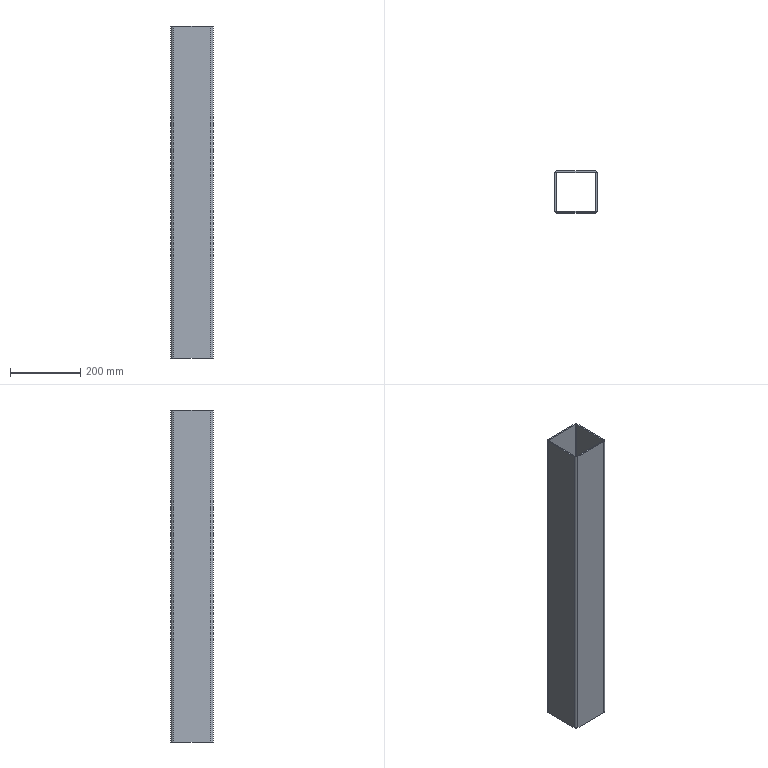Part | SolidWorks | features ICE 1, LibraryFeature 1 | 1 solid | 18 faces | box 120 x 120 x 945 mm | volume 1714983 mm3 | plane 10 | cylinder 8 | commonest cylinder face diameters 8 x4 16 x4
STEP:
#1=CARTESIAN_POINT('',(52.,60.,-472.5));
#2=VERTEX_POINT('',#1);
#3=CARTESIAN_POINT('',(-52.,60.,-472.5));
#4=VERTEX_POINT('',#3);
#5=CARTESIAN_POINT('',(0.,60.,-472.5));
#6=DIRECTION('',(-1.,0.,0.));
#7=VECTOR('',#6,1000.);
#8=LINE('',#5,#7);
#9=EDGE_CURVE('',#2,#4,#8,.T.);
#10=ORIENTED_EDGE('',*,*,#9,.T.);
#11=CARTESIAN_POINT('',(-52.,60.,472.5));
#12=VERTEX_POINT('',#11);
#13=CARTESIAN_POINT('',(-52.,60.,472.5));
#14=DIRECTION('',(0.,0.,-1.));
#15=VECTOR('',#14,1000.);
#16=LINE('',#13,#15);
#17=EDGE_CURVE('',#12,#4,#16,.T.);
#18=ORIENTED_EDGE('',*,*,#17,.F.);
#19=CARTESIAN_POINT('',(52.,60.,472.5));
#20=VERTEX_POINT('',#19);
#21=CARTESIAN_POINT('',(0.,60.,472.5));
#22=DIRECTION('',(-1.,0.,0.));
#23=VECTOR('',#22,1000.);
#24=LINE('',#21,#23);
#25=EDGE_CURVE('',#20,#12,#24,.T.);
#26=ORIENTED_EDGE('',*,*,#25,.F.);
#27=CARTESIAN_POINT('',(52.,60.,472.5));
#28=DIRECTION('',(0.,0.,-1.));
#29=VECTOR('',#28,1000.);
#30=LINE('',#27,#29);
#31=EDGE_CURVE('',#20,#2,#30,.T.);
#32=ORIENTED_EDGE('',*,*,#31,.T.);
#33=EDGE_LOOP('',(#10,#18,#26,#32));
#34=FACE_OUTER_BOUND('',#33,.T.);
#35=CARTESIAN_POINT('',(0.,60.,472.5));
#36=DIRECTION('',(0.,-1.,0.));
#37=DIRECTION('',(0.,0.,-1.));
#38=AXIS2_PLACEMENT_3D('',#35,#36,#37);
#39=PLANE('',#38);
#40=ADVANCED_FACE('',(#34),#39,.F.);
#41=CARTESIAN_POINT('',(-60.,52.,-472.5));
#42=VERTEX_POINT('',#41);
#43=CARTESIAN_POINT('',(-52.,52.,-472.5));
#44=DIRECTION('',(0.,0.,1.));
#45=DIRECTION('',(1.,0.,0.));
#46=AXIS2_PLACEMENT_3D('',#43,#44,#45);
#47=CIRCLE('',#46,8.);
#48=EDGE_CURVE('',#4,#42,#47,.T.);
#49=ORIENTED_EDGE('',*,*,#48,.T.);
#50=CARTESIAN_POINT('',(-60.,52.,472.5));
#51=VERTEX_POINT('',#50);
#52=CARTESIAN_POINT('',(-60.,52.,472.5));
#53=DIRECTION('',(0.,0.,-1.));
#54=VECTOR('',#53,1000.);
#55=LINE('',#52,#54);
#56=EDGE_CURVE('',#51,#42,#55,.T.);
#57=ORIENTED_EDGE('',*,*,#56,.F.);
#58=CARTESIAN_POINT('',(-52.,52.,472.5));
#59=DIRECTION('',(0.,0.,1.));
#60=DIRECTION('',(1.,0.,0.));
#61=AXIS2_PLACEMENT_3D('',#58,#59,#60);
#62=CIRCLE('',#61,8.);
#63=EDGE_CURVE('',#12,#51,#62,.T.);
#64=ORIENTED_EDGE('',*,*,#63,.F.);
#65=ORIENTED_EDGE('',*,*,#17,.T.);
#66=EDGE_LOOP('',(#49,#57,#64,#65));
#67=FACE_OUTER_BOUND('',#66,.T.);
#68=CARTESIAN_POINT('',(-52.,52.,472.5));
#69=DIRECTION('',(0.,0.,-1.));
#70=DIRECTION('',(-1.,0.,0.));
#71=AXIS2_PLACEMENT_3D('',#68,#69,#70);
#72=CYLINDRICAL_SURFACE('',#71,8.);
#73=ADVANCED_FACE('',(#67),#72,.T.);
#74=CARTESIAN_POINT('',(-60.,-52.,-472.5));
#75=VERTEX_POINT('',#74);
#76=CARTESIAN_POINT('',(-60.,0.,-472.5));
#77=DIRECTION('',(0.,1.,0.));
#78=VECTOR('',#77,1000.);
#79=LINE('',#76,#78);
#80=EDGE_CURVE('',#75,#42,#79,.T.);
#81=ORIENTED_EDGE('',*,*,#80,.F.);
#82=CARTESIAN_POINT('',(-60.,-52.,472.5));
#83=VERTEX_POINT('',#82);
#84=CARTESIAN_POINT('',(-60.,-52.,472.5));
#85=DIRECTION('',(0.,0.,-1.));
#86=VECTOR('',#85,1000.);
#87=LINE('',#84,#86);
#88=EDGE_CURVE('',#83,#75,#87,.T.);
#89=ORIENTED_EDGE('',*,*,#88,.F.);
#90=CARTESIAN_POINT('',(-60.,0.,472.5));
#91=DIRECTION('',(0.,1.,0.));
#92=VECTOR('',#91,1000.);
#93=LINE('',#90,#92);
#94=EDGE_CURVE('',#83,#51,#93,.T.);
#95=ORIENTED_EDGE('',*,*,#94,.T.);
#96=ORIENTED_EDGE('',*,*,#56,.T.);
#97=EDGE_LOOP('',(#81,#89,#95,#96));
#98=FACE_OUTER_BOUND('',#97,.T.);
#99=CARTESIAN_POINT('',(-60.,0.,472.5));
#100=DIRECTION('',(-1.,0.,0.));
#101=DIRECTION('',(0.,0.,1.));
#102=AXIS2_PLACEMENT_3D('',#99,#100,#101);
#103=PLANE('',#102);
#104=ADVANCED_FACE('',(#98),#103,.T.);
#105=CARTESIAN_POINT('',(-52.,-60.,-472.5));
#106=VERTEX_POINT('',#105);
#107=CARTESIAN_POINT('',(-52.,-52.,-472.5));
#108=DIRECTION('',(0.,0.,1.));
#109=DIRECTION('',(1.,0.,0.));
#110=AXIS2_PLACEMENT_3D('',#107,#108,#109);
#111=CIRCLE('',#110,8.);
#112=EDGE_CURVE('',#75,#106,#111,.T.);
#113=ORIENTED_EDGE('',*,*,#112,.T.);
#114=CARTESIAN_POINT('',(-52.,-60.,472.5));
#115=VERTEX_POINT('',#114);
#116=CARTESIAN_POINT('',(-52.,-60.,472.5));
#117=DIRECTION('',(0.,0.,-1.));
#118=VECTOR('',#117,1000.);
#119=LINE('',#116,#118);
#120=EDGE_CURVE('',#115,#106,#119,.T.);
#121=ORIENTED_EDGE('',*,*,#120,.F.);
#122=CARTESIAN_POINT('',(-52.,-52.,472.5));
#123=DIRECTION('',(0.,0.,1.));
#124=DIRECTION('',(1.,0.,0.));
#125=AXIS2_PLACEMENT_3D('',#122,#123,#124);
#126=CIRCLE('',#125,8.);
#127=EDGE_CURVE('',#83,#115,#126,.T.);
#128=ORIENTED_EDGE('',*,*,#127,.F.);
#129=ORIENTED_EDGE('',*,*,#88,.T.);
#130=EDGE_LOOP('',(#113,#121,#128,#129));
#131=FACE_OUTER_BOUND('',#130,.T.);
#132=CARTESIAN_POINT('',(-52.,-52.,472.5));
#133=DIRECTION('',(0.,0.,-1.));
#134=DIRECTION('',(-1.,0.,0.));
#135=AXIS2_PLACEMENT_3D('',#132,#133,#134);
#136=CYLINDRICAL_SURFACE('',#135,8.);
#137=ADVANCED_FACE('',(#131),#136,.T.);
#138=CARTESIAN_POINT('',(52.,-60.,-472.5));
#139=VERTEX_POINT('',#138);
#140=CARTESIAN_POINT('',(0.,-60.,-472.5));
#141=DIRECTION('',(1.,0.,0.));
#142=VECTOR('',#141,1000.);
#143=LINE('',#140,#142);
#144=EDGE_CURVE('',#106,#139,#143,.T.);
#145=ORIENTED_EDGE('',*,*,#144,.T.);
#146=CARTESIAN_POINT('',(52.,-60.,472.5));
#147=VERTEX_POINT('',#146);
#148=CARTESIAN_POINT('',(52.,-60.,472.5));
#149=DIRECTION('',(0.,0.,-1.));
#150=VECTOR('',#149,1000.);
#151=LINE('',#148,#150);
#152=EDGE_CURVE('',#147,#139,#151,.T.);
#153=ORIENTED_EDGE('',*,*,#152,.F.);
#154=CARTESIAN_POINT('',(0.,-60.,472.5));
#155=DIRECTION('',(1.,0.,0.));
#156=VECTOR('',#155,1000.);
#157=LINE('',#154,#156);
#158=EDGE_CURVE('',#115,#147,#157,.T.);
#159=ORIENTED_EDGE('',*,*,#158,.F.);
#160=ORIENTED_EDGE('',*,*,#120,.T.);
#161=EDGE_LOOP('',(#145,#153,#159,#160));
#162=FACE_OUTER_BOUND('',#161,.T.);
#163=CARTESIAN_POINT('',(0.,-60.,472.5));
#164=DIRECTION('',(0.,1.,0.));
#165=DIRECTION('',(0.,0.,1.));
#166=AXIS2_PLACEMENT_3D('',#163,#164,#165);
#167=PLANE('',#166);
#168=ADVANCED_FACE('',(#162),#167,.F.);
#169=CARTESIAN_POINT('',(60.,-52.,-472.5));
#170=VERTEX_POINT('',#169);
#171=CARTESIAN_POINT('',(52.,-52.,-472.5));
#172=DIRECTION('',(0.,0.,1.));
#173=DIRECTION('',(1.,0.,0.));
#174=AXIS2_PLACEMENT_3D('',#171,#172,#173);
#175=CIRCLE('',#174,8.);
#176=EDGE_CURVE('',#139,#170,#175,.T.);
#177=ORIENTED_EDGE('',*,*,#176,.T.);
#178=CARTESIAN_POINT('',(60.,-52.,472.5));
#179=VERTEX_POINT('',#178);
#180=CARTESIAN_POINT('',(60.,-52.,472.5));
#181=DIRECTION('',(0.,0.,-1.));
#182=VECTOR('',#181,1000.);
#183=LINE('',#180,#182);
#184=EDGE_CURVE('',#179,#170,#183,.T.);
#185=ORIENTED_EDGE('',*,*,#184,.F.);
#186=CARTESIAN_POINT('',(52.,-52.,472.5));
#187=DIRECTION('',(0.,0.,1.));
#188=DIRECTION('',(1.,0.,0.));
#189=AXIS2_PLACEMENT_3D('',#186,#187,#188);
#190=CIRCLE('',#189,8.);
#191=EDGE_CURVE('',#147,#179,#190,.T.);
#192=ORIENTED_EDGE('',*,*,#191,.F.);
#193=ORIENTED_EDGE('',*,*,#152,.T.);
#194=EDGE_LOOP('',(#177,#185,#192,#193));
#195=FACE_OUTER_BOUND('',#194,.T.);
#196=CARTESIAN_POINT('',(52.,-52.,472.5));
#197=DIRECTION('',(0.,0.,-1.));
#198=DIRECTION('',(-1.,0.,0.));
#199=AXIS2_PLACEMENT_3D('',#196,#197,#198);
#200=CYLINDRICAL_SURFACE('',#199,8.);
#201=ADVANCED_FACE('',(#195),#200,.T.);
#202=CARTESIAN_POINT('',(60.,52.,-472.5));
#203=VERTEX_POINT('',#202);
#204=CARTESIAN_POINT('',(60.,0.,-472.5));
#205=DIRECTION('',(0.,-1.,0.));
#206=VECTOR('',#205,1000.);
#207=LINE('',#204,#206);
#208=EDGE_CURVE('',#203,#170,#207,.T.);
#209=ORIENTED_EDGE('',*,*,#208,.F.);
#210=CARTESIAN_POINT('',(60.,52.,472.5));
#211=VERTEX_POINT('',#210);
#212=CARTESIAN_POINT('',(60.,52.,472.5));
#213=DIRECTION('',(0.,0.,-1.));
#214=VECTOR('',#213,1000.);
#215=LINE('',#212,#214);
#216=EDGE_CURVE('',#211,#203,#215,.T.);
#217=ORIENTED_EDGE('',*,*,#216,.F.);
#218=CARTESIAN_POINT('',(60.,0.,472.5));
#219=DIRECTION('',(0.,-1.,0.));
#220=VECTOR('',#219,1000.);
#221=LINE('',#218,#220);
#222=EDGE_CURVE('',#211,#179,#221,.T.);
#223=ORIENTED_EDGE('',*,*,#222,.T.);
#224=ORIENTED_EDGE('',*,*,#184,.T.);
#225=EDGE_LOOP('',(#209,#217,#223,#224));
#226=FACE_OUTER_BOUND('',#225,.T.);
#227=CARTESIAN_POINT('',(60.,0.,472.5));
#228=DIRECTION('',(1.,0.,0.));
#229=DIRECTION('',(0.,0.,-1.));
#230=AXIS2_PLACEMENT_3D('',#227,#228,#229);
#231=PLANE('',#230);
#232=ADVANCED_FACE('',(#226),#231,.T.);
#233=CARTESIAN_POINT('',(-56.,-52.,-472.5));
#234=VERTEX_POINT('',#233);
#235=CARTESIAN_POINT('',(-52.,-56.,-472.5));
#236=VERTEX_POINT('',#235);
#237=CARTESIAN_POINT('',(-52.,-52.,-472.5));
#238=DIRECTION('',(0.,0.,1.));
#239=DIRECTION('',(1.,0.,0.));
#240=AXIS2_PLACEMENT_3D('',#237,#238,#239);
#241=CIRCLE('',#240,4.);
#242=EDGE_CURVE('',#234,#236,#241,.T.);
#243=ORIENTED_EDGE('',*,*,#242,.F.);
#244=CARTESIAN_POINT('',(-56.,-52.,472.5));
#245=VERTEX_POINT('',#244);
#246=CARTESIAN_POINT('',(-56.,-52.,472.5));
#247=DIRECTION('',(0.,0.,-1.));
#248=VECTOR('',#247,1000.);
#249=LINE('',#246,#248);
#250=EDGE_CURVE('',#245,#234,#249,.T.);
#251=ORIENTED_EDGE('',*,*,#250,.F.);
#252=CARTESIAN_POINT('',(-52.,-56.,472.5));
#253=VERTEX_POINT('',#252);
#254=CARTESIAN_POINT('',(-52.,-52.,472.5));
#255=DIRECTION('',(0.,0.,1.));
#256=DIRECTION('',(1.,0.,0.));
#257=AXIS2_PLACEMENT_3D('',#254,#255,#256);
#258=CIRCLE('',#257,4.);
#259=EDGE_CURVE('',#245,#253,#258,.T.);
#260=ORIENTED_EDGE('',*,*,#259,.T.);
#261=CARTESIAN_POINT('',(-52.,-56.,472.5));
#262=DIRECTION('',(0.,0.,-1.));
#263=VECTOR('',#262,1000.);
#264=LINE('',#261,#263);
#265=EDGE_CURVE('',#253,#236,#264,.T.);
#266=ORIENTED_EDGE('',*,*,#265,.T.);
#267=EDGE_LOOP('',(#243,#251,#260,#266));
#268=FACE_OUTER_BOUND('',#267,.T.);
#269=CARTESIAN_POINT('',(-52.,-52.,472.5));
#270=DIRECTION('',(0.,0.,-1.));
#271=DIRECTION('',(-1.,0.,0.));
#272=AXIS2_PLACEMENT_3D('',#269,#270,#271);
#273=CYLINDRICAL_SURFACE('',#272,4.);
#274=ADVANCED_FACE('',(#268),#273,.F.);
#275=CARTESIAN_POINT('',(-56.,52.,-472.5));
#276=VERTEX_POINT('',#275);
#277=CARTESIAN_POINT('',(-56.,0.,-472.5));
#278=DIRECTION('',(0.,1.,0.));
#279=VECTOR('',#278,1000.);
#280=LINE('',#277,#279);
#281=EDGE_CURVE('',#234,#276,#280,.T.);
#282=ORIENTED_EDGE('',*,*,#281,.T.);
#283=CARTESIAN_POINT('',(-56.,52.,472.5));
#284=VERTEX_POINT('',#283);
#285=CARTESIAN_POINT('',(-56.,52.,472.5));
#286=DIRECTION('',(0.,0.,-1.));
#287=VECTOR('',#286,1000.);
#288=LINE('',#285,#287);
#289=EDGE_CURVE('',#284,#276,#288,.T.);
#290=ORIENTED_EDGE('',*,*,#289,.F.);
#291=CARTESIAN_POINT('',(-56.,0.,472.5));
#292=DIRECTION('',(0.,1.,0.));
#293=VECTOR('',#292,1000.);
#294=LINE('',#291,#293);
#295=EDGE_CURVE('',#245,#284,#294,.T.);
#296=ORIENTED_EDGE('',*,*,#295,.F.);
#297=ORIENTED_EDGE('',*,*,#250,.T.);
#298=EDGE_LOOP('',(#282,#290,#296,#297));
#299=FACE_OUTER_BOUND('',#298,.T.);
#300=CARTESIAN_POINT('',(-56.,0.,472.5));
#301=DIRECTION('',(-1.,0.,0.));
#302=DIRECTION('',(0.,0.,1.));
#303=AXIS2_PLACEMENT_3D('',#300,#301,#302);
#304=PLANE('',#303);
#305=ADVANCED_FACE('',(#299),#304,.F.);
#306=CARTESIAN_POINT('',(-52.,56.,-472.5));
#307=VERTEX_POINT('',#306);
#308=CARTESIAN_POINT('',(-52.,52.,-472.5));
#309=DIRECTION('',(0.,0.,1.));
#310=DIRECTION('',(1.,0.,0.));
#311=AXIS2_PLACEMENT_3D('',#308,#309,#310);
#312=CIRCLE('',#311,4.);
#313=EDGE_CURVE('',#307,#276,#312,.T.);
#314=ORIENTED_EDGE('',*,*,#313,.F.);
#315=CARTESIAN_POINT('',(-52.,56.,472.5));
#316=VERTEX_POINT('',#315);
#317=CARTESIAN_POINT('',(-52.,56.,472.5));
#318=DIRECTION('',(0.,0.,-1.));
#319=VECTOR('',#318,1000.);
#320=LINE('',#317,#319);
#321=EDGE_CURVE('',#316,#307,#320,.T.);
#322=ORIENTED_EDGE('',*,*,#321,.F.);
#323=CARTESIAN_POINT('',(-52.,52.,472.5));
#324=DIRECTION('',(0.,0.,1.));
#325=DIRECTION('',(1.,0.,0.));
#326=AXIS2_PLACEMENT_3D('',#323,#324,#325);
#327=CIRCLE('',#326,4.);
#328=EDGE_CURVE('',#316,#284,#327,.T.);
#329=ORIENTED_EDGE('',*,*,#328,.T.);
#330=ORIENTED_EDGE('',*,*,#289,.T.);
#331=EDGE_LOOP('',(#314,#322,#329,#330));
#332=FACE_OUTER_BOUND('',#331,.T.);
#333=CARTESIAN_POINT('',(-52.,52.,472.5));
#334=DIRECTION('',(0.,0.,-1.));
#335=DIRECTION('',(-1.,0.,0.));
#336=AXIS2_PLACEMENT_3D('',#333,#334,#335);
#337=CYLINDRICAL_SURFACE('',#336,4.);
#338=ADVANCED_FACE('',(#332),#337,.F.);
#339=CARTESIAN_POINT('',(52.,56.,-472.5));
#340=VERTEX_POINT('',#339);
#341=CARTESIAN_POINT('',(0.,56.,-472.5));
#342=DIRECTION('',(-1.,0.,0.));
#343=VECTOR('',#342,1000.);
#344=LINE('',#341,#343);
#345=EDGE_CURVE('',#340,#307,#344,.T.);
#346=ORIENTED_EDGE('',*,*,#345,.F.);
#347=CARTESIAN_POINT('',(52.,56.,472.5));
#348=VERTEX_POINT('',#347);
#349=CARTESIAN_POINT('',(52.,56.,472.5));
#350=DIRECTION('',(0.,0.,-1.));
#351=VECTOR('',#350,1000.);
#352=LINE('',#349,#351);
#353=EDGE_CURVE('',#348,#340,#352,.T.);
#354=ORIENTED_EDGE('',*,*,#353,.F.);
#355=CARTESIAN_POINT('',(0.,56.,472.5));
#356=DIRECTION('',(-1.,0.,0.));
#357=VECTOR('',#356,1000.);
#358=LINE('',#355,#357);
#359=EDGE_CURVE('',#348,#316,#358,.T.);
#360=ORIENTED_EDGE('',*,*,#359,.T.);
#361=ORIENTED_EDGE('',*,*,#321,.T.);
#362=EDGE_LOOP('',(#346,#354,#360,#361));
#363=FACE_OUTER_BOUND('',#362,.T.);
#364=CARTESIAN_POINT('',(0.,56.,472.5));
#365=DIRECTION('',(0.,-1.,0.));
#366=DIRECTION('',(0.,0.,-1.));
#367=AXIS2_PLACEMENT_3D('',#364,#365,#366);
#368=PLANE('',#367);
#369=ADVANCED_FACE('',(#363),#368,.T.);
#370=CARTESIAN_POINT('',(56.,52.,-472.5));
#371=VERTEX_POINT('',#370);
#372=CARTESIAN_POINT('',(52.,52.,-472.5));
#373=DIRECTION('',(0.,0.,1.));
#374=DIRECTION('',(1.,0.,0.));
#375=AXIS2_PLACEMENT_3D('',#372,#373,#374);
#376=CIRCLE('',#375,4.);
#377=EDGE_CURVE('',#371,#340,#376,.T.);
#378=ORIENTED_EDGE('',*,*,#377,.F.);
#379=CARTESIAN_POINT('',(56.,52.,472.5));
#380=VERTEX_POINT('',#379);
#381=CARTESIAN_POINT('',(56.,52.,472.5));
#382=DIRECTION('',(0.,0.,-1.));
#383=VECTOR('',#382,1000.);
#384=LINE('',#381,#383);
#385=EDGE_CURVE('',#380,#371,#384,.T.);
#386=ORIENTED_EDGE('',*,*,#385,.F.);
#387=CARTESIAN_POINT('',(52.,52.,472.5));
#388=DIRECTION('',(0.,0.,1.));
#389=DIRECTION('',(1.,0.,0.));
#390=AXIS2_PLACEMENT_3D('',#387,#388,#389);
#391=CIRCLE('',#390,4.);
#392=EDGE_CURVE('',#380,#348,#391,.T.);
#393=ORIENTED_EDGE('',*,*,#392,.T.);
#394=ORIENTED_EDGE('',*,*,#353,.T.);
#395=EDGE_LOOP('',(#378,#386,#393,#394));
#396=FACE_OUTER_BOUND('',#395,.T.);
#397=CARTESIAN_POINT('',(52.,52.,472.5));
#398=DIRECTION('',(0.,0.,-1.));
#399=DIRECTION('',(-1.,0.,0.));
#400=AXIS2_PLACEMENT_3D('',#397,#398,#399);
#401=CYLINDRICAL_SURFACE('',#400,4.);
#402=ADVANCED_FACE('',(#396),#401,.F.);
#403=CARTESIAN_POINT('',(56.,-52.,-472.5));
#404=VERTEX_POINT('',#403);
#405=CARTESIAN_POINT('',(56.,0.,-472.5));
#406=DIRECTION('',(0.,-1.,0.));
#407=VECTOR('',#406,1000.);
#408=LINE('',#405,#407);
#409=EDGE_CURVE('',#371,#404,#408,.T.);
#410=ORIENTED_EDGE('',*,*,#409,.T.);
#411=CARTESIAN_POINT('',(56.,-52.,472.5));
#412=VERTEX_POINT('',#411);
#413=CARTESIAN_POINT('',(56.,-52.,472.5));
#414=DIRECTION('',(0.,0.,-1.));
#415=VECTOR('',#414,1000.);
#416=LINE('',#413,#415);
#417=EDGE_CURVE('',#412,#404,#416,.T.);
#418=ORIENTED_EDGE('',*,*,#417,.F.);
#419=CARTESIAN_POINT('',(56.,0.,472.5));
#420=DIRECTION('',(0.,-1.,0.));
#421=VECTOR('',#420,1000.);
#422=LINE('',#419,#421);
#423=EDGE_CURVE('',#380,#412,#422,.T.);
#424=ORIENTED_EDGE('',*,*,#423,.F.);
#425=ORIENTED_EDGE('',*,*,#385,.T.);
#426=EDGE_LOOP('',(#410,#418,#424,#425));
#427=FACE_OUTER_BOUND('',#426,.T.);
#428=CARTESIAN_POINT('',(56.,0.,472.5));
#429=DIRECTION('',(1.,0.,0.));
#430=DIRECTION('',(0.,0.,-1.));
#431=AXIS2_PLACEMENT_3D('',#428,#429,#430);
#432=PLANE('',#431);
#433=ADVANCED_FACE('',(#427),#432,.F.);
#434=CARTESIAN_POINT('',(52.,-56.,-472.5));
#435=VERTEX_POINT('',#434);
#436=CARTESIAN_POINT('',(52.,-52.,-472.5));
#437=DIRECTION('',(0.,0.,1.));
#438=DIRECTION('',(1.,0.,0.));
#439=AXIS2_PLACEMENT_3D('',#436,#437,#438);
#440=CIRCLE('',#439,4.);
#441=EDGE_CURVE('',#435,#404,#440,.T.);
#442=ORIENTED_EDGE('',*,*,#441,.F.);
#443=CARTESIAN_POINT('',(52.,-56.,472.5));
#444=VERTEX_POINT('',#443);
#445=CARTESIAN_POINT('',(52.,-56.,472.5));
#446=DIRECTION('',(0.,0.,-1.));
#447=VECTOR('',#446,1000.);
#448=LINE('',#445,#447);
#449=EDGE_CURVE('',#444,#435,#448,.T.);
#450=ORIENTED_EDGE('',*,*,#449,.F.);
#451=CARTESIAN_POINT('',(52.,-52.,472.5));
#452=DIRECTION('',(0.,0.,1.));
#453=DIRECTION('',(1.,0.,0.));
#454=AXIS2_PLACEMENT_3D('',#451,#452,#453);
#455=CIRCLE('',#454,4.);
#456=EDGE_CURVE('',#444,#412,#455,.T.);
#457=ORIENTED_EDGE('',*,*,#456,.T.);
#458=ORIENTED_EDGE('',*,*,#417,.T.);
#459=EDGE_LOOP('',(#442,#450,#457,#458));
#460=FACE_OUTER_BOUND('',#459,.T.);
#461=CARTESIAN_POINT('',(52.,-52.,472.5));
#462=DIRECTION('',(0.,0.,-1.));
#463=DIRECTION('',(-1.,0.,0.));
#464=AXIS2_PLACEMENT_3D('',#461,#462,#463);
#465=CYLINDRICAL_SURFACE('',#464,4.);
#466=ADVANCED_FACE('',(#460),#465,.F.);
#467=CARTESIAN_POINT('',(0.,-56.,-472.5));
#468=DIRECTION('',(1.,0.,0.));
#469=VECTOR('',#468,1000.);
#470=LINE('',#467,#469);
#471=EDGE_CURVE('',#236,#435,#470,.T.);
#472=ORIENTED_EDGE('',*,*,#471,.F.);
#473=ORIENTED_EDGE('',*,*,#265,.F.);
#474=CARTESIAN_POINT('',(0.,-56.,472.5));
#475=DIRECTION('',(1.,0.,0.));
#476=VECTOR('',#475,1000.);
#477=LINE('',#474,#476);
#478=EDGE_CURVE('',#253,#444,#477,.T.);
#479=ORIENTED_EDGE('',*,*,#478,.T.);
#480=ORIENTED_EDGE('',*,*,#449,.T.);
#481=EDGE_LOOP('',(#472,#473,#479,#480));
#482=FACE_OUTER_BOUND('',#481,.T.);
#483=CARTESIAN_POINT('',(0.,-56.,472.5));
#484=DIRECTION('',(0.,1.,0.));
#485=DIRECTION('',(0.,0.,1.));
#486=AXIS2_PLACEMENT_3D('',#483,#484,#485);
#487=PLANE('',#486);
#488=ADVANCED_FACE('',(#482),#487,.T.);
#489=CARTESIAN_POINT('',(52.,52.,-472.5));
#490=DIRECTION('',(0.,0.,1.));
#491=DIRECTION('',(1.,0.,0.));
#492=AXIS2_PLACEMENT_3D('',#489,#490,#491);
#493=CIRCLE('',#492,8.);
#494=EDGE_CURVE('',#203,#2,#493,.T.);
#495=ORIENTED_EDGE('',*,*,#494,.T.);
#496=ORIENTED_EDGE('',*,*,#31,.F.);
#497=CARTESIAN_POINT('',(52.,52.,472.5));
#498=DIRECTION('',(0.,0.,1.));
#499=DIRECTION('',(1.,0.,0.));
#500=AXIS2_PLACEMENT_3D('',#497,#498,#499);
#501=CIRCLE('',#500,8.);
#502=EDGE_CURVE('',#211,#20,#501,.T.);
#503=ORIENTED_EDGE('',*,*,#502,.F.);
#504=ORIENTED_EDGE('',*,*,#216,.T.);
#505=EDGE_LOOP('',(#495,#496,#503,#504));
#506=FACE_OUTER_BOUND('',#505,.T.);
#507=CARTESIAN_POINT('',(52.,52.,472.5));
#508=DIRECTION('',(0.,0.,-1.));
#509=DIRECTION('',(-1.,0.,0.));
#510=AXIS2_PLACEMENT_3D('',#507,#508,#509);
#511=CYLINDRICAL_SURFACE('',#510,8.);
#512=ADVANCED_FACE('',(#506),#511,.T.);
#513=ORIENTED_EDGE('',*,*,#259,.F.);
#514=ORIENTED_EDGE('',*,*,#295,.T.);
#515=ORIENTED_EDGE('',*,*,#328,.F.);
#516=ORIENTED_EDGE('',*,*,#359,.F.);
#517=ORIENTED_EDGE('',*,*,#392,.F.);
#518=ORIENTED_EDGE('',*,*,#423,.T.);
#519=ORIENTED_EDGE('',*,*,#456,.F.);
#520=ORIENTED_EDGE('',*,*,#478,.F.);
#521=EDGE_LOOP('',(#513,#514,#515,#516,#517,#518,#519,#520));
#522=FACE_BOUND('',#521,.T.);
#523=ORIENTED_EDGE('',*,*,#25,.T.);
#524=ORIENTED_EDGE('',*,*,#63,.T.);
#525=ORIENTED_EDGE('',*,*,#94,.F.);
#526=ORIENTED_EDGE('',*,*,#127,.T.);
#527=ORIENTED_EDGE('',*,*,#158,.T.);
#528=ORIENTED_EDGE('',*,*,#191,.T.);
#529=ORIENTED_EDGE('',*,*,#222,.F.);
#530=ORIENTED_EDGE('',*,*,#502,.T.);
#531=EDGE_LOOP('',(#523,#524,#525,#526,#527,#528,#529,#530));
#532=FACE_OUTER_BOUND('',#531,.T.);
#533=CARTESIAN_POINT('',(0.,0.,472.5));
#534=DIRECTION('',(0.,0.,1.));
#535=DIRECTION('',(1.,0.,0.));
#536=AXIS2_PLACEMENT_3D('',#533,#534,#535);
#537=PLANE('',#536);
#538=ADVANCED_FACE('',(#522,#532),#537,.T.);
#539=ORIENTED_EDGE('',*,*,#242,.T.);
#540=ORIENTED_EDGE('',*,*,#471,.T.);
#541=ORIENTED_EDGE('',*,*,#441,.T.);
#542=ORIENTED_EDGE('',*,*,#409,.F.);
#543=ORIENTED_EDGE('',*,*,#377,.T.);
#544=ORIENTED_EDGE('',*,*,#345,.T.);
#545=ORIENTED_EDGE('',*,*,#313,.T.);
#546=ORIENTED_EDGE('',*,*,#281,.F.);
#547=EDGE_LOOP('',(#539,#540,#541,#542,#543,#544,#545,#546));
#548=FACE_BOUND('',#547,.T.);
#549=ORIENTED_EDGE('',*,*,#9,.F.);
#550=ORIENTED_EDGE('',*,*,#494,.F.);
#551=ORIENTED_EDGE('',*,*,#208,.T.);
#552=ORIENTED_EDGE('',*,*,#176,.F.);
#553=ORIENTED_EDGE('',*,*,#144,.F.);
#554=ORIENTED_EDGE('',*,*,#112,.F.);
#555=ORIENTED_EDGE('',*,*,#80,.T.);
#556=ORIENTED_EDGE('',*,*,#48,.F.);
#557=EDGE_LOOP('',(#549,#550,#551,#552,#553,#554,#555,#556));
#558=FACE_OUTER_BOUND('',#557,.T.);
#559=CARTESIAN_POINT('',(0.,0.,-472.5));
#560=DIRECTION('',(0.,0.,1.));
#561=DIRECTION('',(1.,0.,0.));
#562=AXIS2_PLACEMENT_3D('',#559,#560,#561);
#563=PLANE('',#562);
#564=ADVANCED_FACE('',(#548,#558),#563,.F.);
#565=CLOSED_SHELL('',(#40,#73,#104,#137,#168,#201,#232,#274,#305,#338,#369,#402,#433,#466,#488,#512,#538,#564));
#566=MANIFOLD_SOLID_BREP('',#565);
#567=CARTESIAN_POINT('',(0.,0.,0.));
#568=DIRECTION('',(0.,0.,1.));
#569=DIRECTION('',(1.,0.,0.));
#570=AXIS2_PLACEMENT_3D('',#567,#568,#569);
#571=(LENGTH_UNIT()NAMED_UNIT(*)SI_UNIT(.MILLI.,.METRE.));
#572=UNCERTAINTY_MEASURE_WITH_UNIT(LENGTH_MEASURE(0.00001),#571,'','');
#573=(NAMED_UNIT(*)PLANE_ANGLE_UNIT()SI_UNIT($,.RADIAN.));
#574=(NAMED_UNIT(*)SI_UNIT($,.STERADIAN.)SOLID_ANGLE_UNIT());
#575=(GEOMETRIC_REPRESENTATION_CONTEXT(3)GLOBAL_UNCERTAINTY_ASSIGNED_CONTEXT((#572))GLOBAL_UNIT_ASSIGNED_CONTEXT((#571,#573,#574))REPRESENTATION_CONTEXT('',''));
#576=ADVANCED_BREP_SHAPE_REPRESENTATION('',(#566,#570),#575);